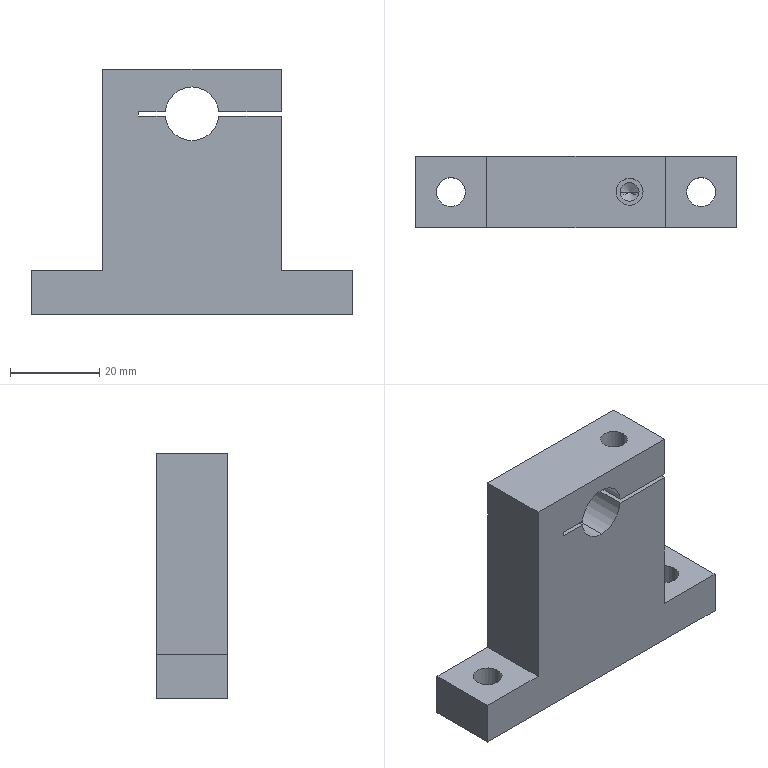Part | STEP file | 0232_204_Holder | 1 solid | 29 faces | box 72 x 16 x 55 mm | volume 37017 mm3 | plane 16 | cylinder 11 | cone 2 | commonest cylinder face diameters 6.5 x4 12 x3 4.2 x2 6 x2